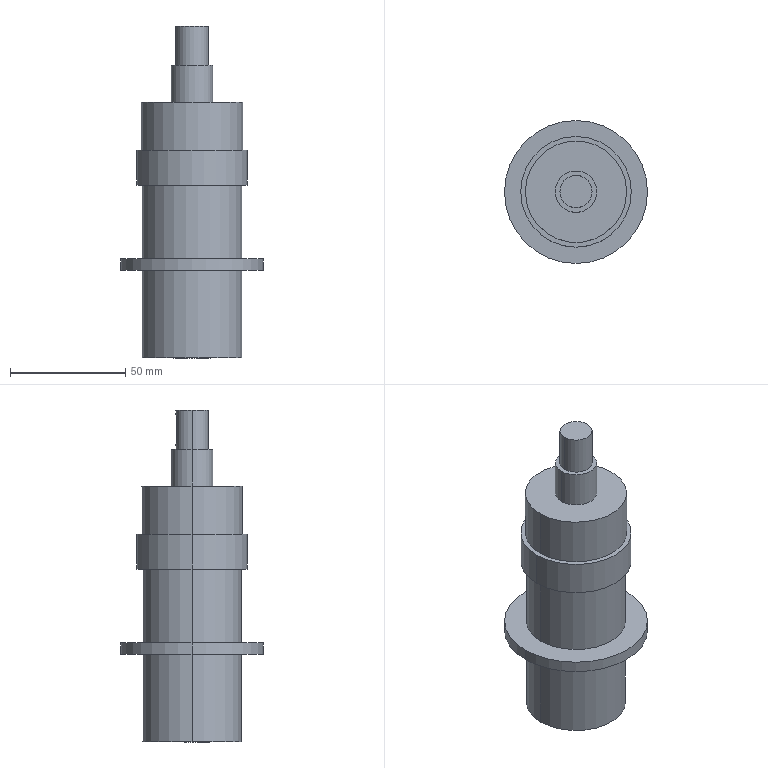Part | SolidWorks | features ICE 6, 3DProfileFeature 1, Cut 1, Extrusion 1, HoleWzd 1 | 1 solid | 32 faces | box 62 x 62 x 144 mm | volume 181126 mm3 | cylinder 19 | plane 11 | cone 2 | commonest cylinder face diameters 43 x4 3.7 x3 6.8 x2 14 x2 18 x2 44 x2
STEP:
#1=CARTESIAN_POINT('',(3.4,0.,35.));
#2=VERTEX_POINT('',#1);
#3=CARTESIAN_POINT('',(-3.4,0.,35.));
#4=VERTEX_POINT('',#3);
#5=CARTESIAN_POINT('',(0.,0.,35.));
#6=DIRECTION('',(0.,0.,-1.));
#7=DIRECTION('',(-1.,0.,0.));
#8=AXIS2_PLACEMENT_3D('',#5,#6,#7);
#9=CIRCLE('',#8,3.4);
#10=EDGE_CURVE('',#2,#4,#9,.T.);
#11=ORIENTED_EDGE('',*,*,#10,.F.);
#12=CARTESIAN_POINT('',(3.4,0.,0.));
#13=VERTEX_POINT('',#12);
#14=CARTESIAN_POINT('',(3.4,0.,0.));
#15=DIRECTION('',(0.,0.,-1.));
#16=VECTOR('',#15,1000.);
#17=LINE('',#14,#16);
#18=EDGE_CURVE('',#2,#13,#17,.T.);
#19=ORIENTED_EDGE('',*,*,#18,.T.);
#20=CARTESIAN_POINT('',(-3.4,0.,0.));
#21=VERTEX_POINT('',#20);
#22=CARTESIAN_POINT('',(0.,0.,0.));
#23=DIRECTION('',(0.,0.,-1.));
#24=DIRECTION('',(-1.,0.,0.));
#25=AXIS2_PLACEMENT_3D('',#22,#23,#24);
#26=CIRCLE('',#25,3.4);
#27=EDGE_CURVE('',#13,#21,#26,.T.);
#28=ORIENTED_EDGE('',*,*,#27,.T.);
#29=CARTESIAN_POINT('',(-3.4,0.,0.));
#30=DIRECTION('',(0.,0.,-1.));
#31=VECTOR('',#30,1000.);
#32=LINE('',#29,#31);
#33=EDGE_CURVE('',#4,#21,#32,.T.);
#34=ORIENTED_EDGE('',*,*,#33,.F.);
#35=EDGE_LOOP('',(#11,#19,#28,#34));
#36=FACE_OUTER_BOUND('',#35,.T.);
#37=CARTESIAN_POINT('',(0.,0.,0.));
#38=DIRECTION('',(0.,0.,-1.));
#39=DIRECTION('',(-1.,0.,0.));
#40=AXIS2_PLACEMENT_3D('',#37,#38,#39);
#41=CYLINDRICAL_SURFACE('',#40,3.4);
#42=ADVANCED_FACE('',(#36),#41,.F.);
#43=CARTESIAN_POINT('',(0.,0.,37.043));
#44=VERTEX_POINT('',#43);
#45=CARTESIAN_POINT('',(-3.4,0.,35.));
#46=DIRECTION('',(-0.8572,0.,-0.515));
#47=VECTOR('',#46,1000.);
#48=LINE('',#45,#47);
#49=EDGE_CURVE('',#44,#4,#48,.T.);
#50=ORIENTED_EDGE('',*,*,#49,.F.);
#51=CARTESIAN_POINT('',(3.4,0.,35.));
#52=DIRECTION('',(0.8572,0.,-0.515));
#53=VECTOR('',#52,1000.);
#54=LINE('',#51,#53);
#55=EDGE_CURVE('',#44,#2,#54,.T.);
#56=ORIENTED_EDGE('',*,*,#55,.T.);
#57=ORIENTED_EDGE('',*,*,#10,.T.);
#58=EDGE_LOOP('',(#50,#56,#57));
#59=FACE_OUTER_BOUND('',#58,.T.);
#60=CARTESIAN_POINT('',(0.,0.,35.));
#61=DIRECTION('',(0.,0.,-1.));
#62=DIRECTION('',(-1.,0.,0.));
#63=AXIS2_PLACEMENT_3D('',#60,#61,#62);
#64=CONICAL_SURFACE('',#63,3.4,1.03);
#65=ADVANCED_FACE('',(#59),#64,.F.);
#66=CARTESIAN_POINT('',(21.5,0.,38.));
#67=VERTEX_POINT('',#66);
#68=CARTESIAN_POINT('',(-21.5,0.,38.));
#69=VERTEX_POINT('',#68);
#70=CARTESIAN_POINT('',(0.,0.,38.));
#71=DIRECTION('',(0.,0.,1.));
#72=DIRECTION('',(1.,0.,0.));
#73=AXIS2_PLACEMENT_3D('',#70,#71,#72);
#74=CIRCLE('',#73,21.5);
#75=EDGE_CURVE('',#67,#69,#74,.T.);
#76=ORIENTED_EDGE('',*,*,#75,.F.);
#77=CARTESIAN_POINT('',(21.5,0.,0.));
#78=VERTEX_POINT('',#77);
#79=CARTESIAN_POINT('',(21.5,0.,75.));
#80=DIRECTION('',(0.,0.,-1.));
#81=VECTOR('',#80,1000.);
#82=LINE('',#79,#81);
#83=EDGE_CURVE('',#67,#78,#82,.T.);
#84=ORIENTED_EDGE('',*,*,#83,.T.);
#85=CARTESIAN_POINT('',(-21.5,0.,0.));
#86=VERTEX_POINT('',#85);
#87=CARTESIAN_POINT('',(0.,0.,0.));
#88=DIRECTION('',(0.,0.,-1.));
#89=DIRECTION('',(-1.,0.,0.));
#90=AXIS2_PLACEMENT_3D('',#87,#88,#89);
#91=CIRCLE('',#90,21.5);
#92=EDGE_CURVE('',#86,#78,#91,.T.);
#93=ORIENTED_EDGE('',*,*,#92,.F.);
#94=CARTESIAN_POINT('',(-21.5,0.,75.));
#95=DIRECTION('',(0.,0.,-1.));
#96=VECTOR('',#95,1000.);
#97=LINE('',#94,#96);
#98=EDGE_CURVE('',#69,#86,#97,.T.);
#99=ORIENTED_EDGE('',*,*,#98,.F.);
#100=EDGE_LOOP('',(#76,#84,#93,#99));
#101=FACE_OUTER_BOUND('',#100,.T.);
#102=CARTESIAN_POINT('',(0.,0.,75.));
#103=DIRECTION('',(0.,0.,-1.));
#104=DIRECTION('',(-1.,0.,0.));
#105=AXIS2_PLACEMENT_3D('',#102,#103,#104);
#106=CYLINDRICAL_SURFACE('',#105,21.5);
#107=ADVANCED_FACE('',(#101),#106,.T.);
#108=CARTESIAN_POINT('',(31.,0.,43.));
#109=VERTEX_POINT('',#108);
#110=CARTESIAN_POINT('',(-31.,0.,43.));
#111=VERTEX_POINT('',#110);
#112=CARTESIAN_POINT('',(0.,0.,43.));
#113=DIRECTION('',(0.,0.,1.));
#114=DIRECTION('',(1.,0.,0.));
#115=AXIS2_PLACEMENT_3D('',#112,#113,#114);
#116=CIRCLE('',#115,31.);
#117=EDGE_CURVE('',#109,#111,#116,.T.);
#118=ORIENTED_EDGE('',*,*,#117,.F.);
#119=CARTESIAN_POINT('',(31.,0.,38.));
#120=VERTEX_POINT('',#119);
#121=CARTESIAN_POINT('',(31.,0.,43.));
#122=DIRECTION('',(0.,0.,-1.));
#123=VECTOR('',#122,1000.);
#124=LINE('',#121,#123);
#125=EDGE_CURVE('',#109,#120,#124,.T.);
#126=ORIENTED_EDGE('',*,*,#125,.T.);
#127=CARTESIAN_POINT('',(-31.,0.,38.));
#128=VERTEX_POINT('',#127);
#129=CARTESIAN_POINT('',(0.,0.,38.));
#130=DIRECTION('',(0.,0.,1.));
#131=DIRECTION('',(1.,0.,0.));
#132=AXIS2_PLACEMENT_3D('',#129,#130,#131);
#133=CIRCLE('',#132,31.);
#134=EDGE_CURVE('',#120,#128,#133,.T.);
#135=ORIENTED_EDGE('',*,*,#134,.T.);
#136=CARTESIAN_POINT('',(-31.,0.,43.));
#137=DIRECTION('',(0.,0.,-1.));
#138=VECTOR('',#137,1000.);
#139=LINE('',#136,#138);
#140=EDGE_CURVE('',#111,#128,#139,.T.);
#141=ORIENTED_EDGE('',*,*,#140,.F.);
#142=EDGE_LOOP('',(#118,#126,#135,#141));
#143=FACE_OUTER_BOUND('',#142,.T.);
#144=CARTESIAN_POINT('',(0.,0.,43.));
#145=DIRECTION('',(0.,0.,-1.));
#146=DIRECTION('',(-1.,0.,0.));
#147=AXIS2_PLACEMENT_3D('',#144,#145,#146);
#148=CYLINDRICAL_SURFACE('',#147,31.);
#149=ADVANCED_FACE('',(#143),#148,.T.);
#150=CARTESIAN_POINT('',(0.,5.,142.35));
#151=VERTEX_POINT('',#150);
#152=CARTESIAN_POINT('',(1.85,5.,140.5));
#153=VERTEX_POINT('',#152);
#154=CARTESIAN_POINT('',(0.,5.,140.5));
#155=DIRECTION('',(0.,1.,0.));
#156=DIRECTION('',(0.,0.,1.));
#157=AXIS2_PLACEMENT_3D('',#154,#155,#156);
#158=CIRCLE('',#157,1.85);
#159=EDGE_CURVE('',#151,#153,#158,.T.);
#160=ORIENTED_EDGE('',*,*,#159,.F.);
#161=CARTESIAN_POINT('',(0.,7.,142.35));
#162=VERTEX_POINT('',#161);
#163=CARTESIAN_POINT('',(0.,5.,142.35));
#164=DIRECTION('',(0.,1.,0.));
#165=VECTOR('',#164,1000.);
#166=LINE('',#163,#165);
#167=EDGE_CURVE('',#151,#162,#166,.T.);
#168=ORIENTED_EDGE('',*,*,#167,.T.);
#169=CARTESIAN_POINT('',(1.85,6.751,140.5));
#170=VERTEX_POINT('',#169);
#171=CARTESIAN_POINT('',(1.85,6.751,140.5));
#172=CARTESIAN_POINT('',(1.85,6.751,140.623));
#173=CARTESIAN_POINT('',(1.838,6.754,140.744));
#174=CARTESIAN_POINT('',(1.791,6.767,140.981));
#175=CARTESIAN_POINT('',(1.755,6.777,141.099));
#176=CARTESIAN_POINT('',(1.662,6.8,141.322));
#177=CARTESIAN_POINT('',(1.605,6.814,141.429));
#178=CARTESIAN_POINT('',(1.47,6.844,141.629));
#179=CARTESIAN_POINT('',(1.393,6.861,141.724));
#180=CARTESIAN_POINT('',(1.138,6.909,141.979));
#181=CARTESIAN_POINT('',(0.932,6.941,142.116));
#182=CARTESIAN_POINT('',(0.5982,6.975,142.255));
#183=CARTESIAN_POINT('',(0.4809,6.984,142.291));
#184=CARTESIAN_POINT('',(0.2418,6.997,142.338));
#185=CARTESIAN_POINT('',(0.1213,7.,142.35));
#186=CARTESIAN_POINT('',(0.,7.,142.35));
#187=B_SPLINE_CURVE_WITH_KNOTS('',3,(#171,#172,#173,#174,#175,#176,#177,#178,#179,#180,#181,#182,#183,#184,#185,#186),.UNSPECIFIED.,.F.,.F.,(4,2,2,2,2,2,2,4),(0.,0.0003632,0.0007264,0.00109,0.001453,0.002179,0.002542,0.002906),.UNSPECIFIED.);
#188=EDGE_CURVE('',#170,#162,#187,.T.);
#189=ORIENTED_EDGE('',*,*,#188,.F.);
#190=CARTESIAN_POINT('',(1.85,5.,140.5));
#191=DIRECTION('',(0.,1.,0.));
#192=VECTOR('',#191,1000.);
#193=LINE('',#190,#192);
#194=EDGE_CURVE('',#153,#170,#193,.T.);
#195=ORIENTED_EDGE('',*,*,#194,.F.);
#196=EDGE_LOOP('',(#160,#168,#189,#195));
#197=FACE_OUTER_BOUND('',#196,.T.);
#198=CARTESIAN_POINT('',(0.,5.,140.5));
#199=DIRECTION('',(0.,1.,0.));
#200=DIRECTION('',(0.,0.,1.));
#201=AXIS2_PLACEMENT_3D('',#198,#199,#200);
#202=CYLINDRICAL_SURFACE('',#201,1.85);
#203=ADVANCED_FACE('',(#197),#202,.F.);
#204=CARTESIAN_POINT('',(-1.85,6.751,140.5));
#205=VERTEX_POINT('',#204);
#206=CARTESIAN_POINT('',(-1.85,6.751,130.64));
#207=VERTEX_POINT('',#206);
#208=CARTESIAN_POINT('',(-1.85,6.751,144.));
#209=DIRECTION('',(0.,0.,-1.));
#210=VECTOR('',#209,1000.);
#211=LINE('',#208,#210);
#212=EDGE_CURVE('',#205,#207,#211,.T.);
#213=ORIENTED_EDGE('',*,*,#212,.T.);
#214=CARTESIAN_POINT('',(1.85,6.751,130.64));
#215=VERTEX_POINT('',#214);
#216=CARTESIAN_POINT('',(-1.85,6.751,130.64));
#217=CARTESIAN_POINT('',(-1.85,6.751,130.517));
#218=CARTESIAN_POINT('',(-1.838,6.754,130.397));
#219=CARTESIAN_POINT('',(-1.791,6.767,130.159));
#220=CARTESIAN_POINT('',(-1.755,6.777,130.042));
#221=CARTESIAN_POINT('',(-1.662,6.8,129.818));
#222=CARTESIAN_POINT('',(-1.605,6.814,129.712));
#223=CARTESIAN_POINT('',(-1.471,6.844,129.511));
#224=CARTESIAN_POINT('',(-1.393,6.861,129.417));
#225=CARTESIAN_POINT('',(-1.138,6.909,129.162));
#226=CARTESIAN_POINT('',(-0.933,6.941,129.024));
#227=CARTESIAN_POINT('',(-0.5995,6.975,128.886));
#228=CARTESIAN_POINT('',(-0.4823,6.984,128.85));
#229=CARTESIAN_POINT('',(-0.2433,6.997,128.802));
#230=CARTESIAN_POINT('',(-0.1229,7.,128.79));
#231=CARTESIAN_POINT('',(0.1195,7.,128.79));
#232=CARTESIAN_POINT('',(0.2427,6.997,128.802));
#233=CARTESIAN_POINT('',(0.4804,6.985,128.849));
#234=CARTESIAN_POINT('',(0.596,6.975,128.884));
#235=CARTESIAN_POINT('',(0.933,6.941,129.024));
#236=CARTESIAN_POINT('',(1.136,6.909,129.16));
#237=CARTESIAN_POINT('',(1.393,6.86,129.417));
#238=CARTESIAN_POINT('',(1.469,6.844,129.51));
#239=CARTESIAN_POINT('',(1.603,6.814,129.709));
#240=CARTESIAN_POINT('',(1.662,6.8,129.818));
#241=CARTESIAN_POINT('',(1.801,6.765,130.152));
#242=CARTESIAN_POINT('',(1.85,6.751,130.394));
#243=CARTESIAN_POINT('',(1.85,6.751,130.64));
#244=B_SPLINE_CURVE_WITH_KNOTS('',3,(#216,#217,#218,#219,#220,#221,#222,#223,#224,#225,#226,#227,#228,#229,#230,#231,#232,#233,#234,#235,#236,#237,#238,#239,#240,#241,#242,#243),.UNSPECIFIED.,.F.,.F.,(4,2,2,2,2,2,2,2,2,2,2,2,2,4),(0.,0.000363,0.000726,0.001089,0.001452,0.002178,0.002541,0.002904,0.003267,0.00363,0.004356,0.004719,0.005082,0.005808),.UNSPECIFIED.);
#245=EDGE_CURVE('',#207,#215,#244,.T.);
#246=ORIENTED_EDGE('',*,*,#245,.T.);
#247=CARTESIAN_POINT('',(1.85,6.751,144.));
#248=DIRECTION('',(0.,0.,1.));
#249=VECTOR('',#248,1000.);
#250=LINE('',#247,#249);
#251=EDGE_CURVE('',#215,#170,#250,.T.);
#252=ORIENTED_EDGE('',*,*,#251,.T.);
#253=ORIENTED_EDGE('',*,*,#188,.T.);
#254=CARTESIAN_POINT('',(0.,7.,142.35));
#255=CARTESIAN_POINT('',(-0.1212,7.,142.35));
#256=CARTESIAN_POINT('',(-0.2443,6.997,142.338));
#257=CARTESIAN_POINT('',(-0.4818,6.984,142.29));
#258=CARTESIAN_POINT('',(-0.5973,6.975,142.255));
#259=CARTESIAN_POINT('',(-0.934,6.941,142.115));
#260=CARTESIAN_POINT('',(-1.137,6.909,141.979));
#261=CARTESIAN_POINT('',(-1.394,6.86,141.723));
#262=CARTESIAN_POINT('',(-1.47,6.844,141.63));
#263=CARTESIAN_POINT('',(-1.604,6.814,141.43));
#264=CARTESIAN_POINT('',(-1.662,6.8,141.322));
#265=CARTESIAN_POINT('',(-1.801,6.765,140.987));
#266=CARTESIAN_POINT('',(-1.85,6.751,140.745));
#267=CARTESIAN_POINT('',(-1.85,6.751,140.5));
#268=B_SPLINE_CURVE_WITH_KNOTS('',3,(#254,#255,#256,#257,#258,#259,#260,#261,#262,#263,#264,#265,#266,#267),.UNSPECIFIED.,.F.,.F.,(4,2,2,2,2,2,4),(0.002906,0.003268,0.003631,0.004357,0.00472,0.005082,0.005808),.UNSPECIFIED.);
#269=EDGE_CURVE('',#162,#205,#268,.T.);
#270=ORIENTED_EDGE('',*,*,#269,.T.);
#271=EDGE_LOOP('',(#213,#246,#252,#253,#270));
#272=FACE_BOUND('',#271,.T.);
#273=CARTESIAN_POINT('',(7.,0.,144.));
#274=VERTEX_POINT('',#273);
#275=CARTESIAN_POINT('',(-7.,0.,144.));
#276=VERTEX_POINT('',#275);
#277=CARTESIAN_POINT('',(0.,0.,144.));
#278=DIRECTION('',(0.,0.,1.));
#279=DIRECTION('',(1.,0.,0.));
#280=AXIS2_PLACEMENT_3D('',#277,#278,#279);
#281=CIRCLE('',#280,7.);
#282=EDGE_CURVE('',#274,#276,#281,.T.);
#283=ORIENTED_EDGE('',*,*,#282,.F.);
#284=CARTESIAN_POINT('',(7.,0.,127.));
#285=VERTEX_POINT('',#284);
#286=CARTESIAN_POINT('',(7.,0.,144.));
#287=DIRECTION('',(0.,0.,-1.));
#288=VECTOR('',#287,1000.);
#289=LINE('',#286,#288);
#290=EDGE_CURVE('',#274,#285,#289,.T.);
#291=ORIENTED_EDGE('',*,*,#290,.T.);
#292=CARTESIAN_POINT('',(-7.,0.,127.));
#293=VERTEX_POINT('',#292);
#294=CARTESIAN_POINT('',(0.,0.,127.));
#295=DIRECTION('',(0.,0.,1.));
#296=DIRECTION('',(1.,0.,0.));
#297=AXIS2_PLACEMENT_3D('',#294,#295,#296);
#298=CIRCLE('',#297,7.);
#299=EDGE_CURVE('',#285,#293,#298,.T.);
#300=ORIENTED_EDGE('',*,*,#299,.T.);
#301=CARTESIAN_POINT('',(-7.,0.,144.));
#302=DIRECTION('',(0.,0.,-1.));
#303=VECTOR('',#302,1000.);
#304=LINE('',#301,#303);
#305=EDGE_CURVE('',#276,#293,#304,.T.);
#306=ORIENTED_EDGE('',*,*,#305,.F.);
#307=EDGE_LOOP('',(#283,#291,#300,#306));
#308=FACE_OUTER_BOUND('',#307,.T.);
#309=CARTESIAN_POINT('',(0.,0.,144.));
#310=DIRECTION('',(0.,0.,-1.));
#311=DIRECTION('',(-1.,0.,0.));
#312=AXIS2_PLACEMENT_3D('',#309,#310,#311);
#313=CYLINDRICAL_SURFACE('',#312,7.);
#314=ADVANCED_FACE('',(#272,#308),#313,.T.);
#315=CARTESIAN_POINT('',(9.,0.,127.));
#316=VERTEX_POINT('',#315);
#317=CARTESIAN_POINT('',(-9.,0.,127.));
#318=VERTEX_POINT('',#317);
#319=CARTESIAN_POINT('',(0.,0.,127.));
#320=DIRECTION('',(0.,0.,1.));
#321=DIRECTION('',(1.,0.,0.));
#322=AXIS2_PLACEMENT_3D('',#319,#320,#321);
#323=CIRCLE('',#322,9.);
#324=EDGE_CURVE('',#316,#318,#323,.T.);
#325=ORIENTED_EDGE('',*,*,#324,.F.);
#326=CARTESIAN_POINT('',(9.,0.,111.));
#327=VERTEX_POINT('',#326);
#328=CARTESIAN_POINT('',(9.,0.,127.));
#329=DIRECTION('',(0.,0.,-1.));
#330=VECTOR('',#329,1000.);
#331=LINE('',#328,#330);
#332=EDGE_CURVE('',#316,#327,#331,.T.);
#333=ORIENTED_EDGE('',*,*,#332,.T.);
#334=CARTESIAN_POINT('',(-9.,0.,111.));
#335=VERTEX_POINT('',#334);
#336=CARTESIAN_POINT('',(0.,0.,111.));
#337=DIRECTION('',(0.,0.,1.));
#338=DIRECTION('',(1.,0.,0.));
#339=AXIS2_PLACEMENT_3D('',#336,#337,#338);
#340=CIRCLE('',#339,9.);
#341=EDGE_CURVE('',#327,#335,#340,.T.);
#342=ORIENTED_EDGE('',*,*,#341,.T.);
#343=CARTESIAN_POINT('',(-9.,0.,127.));
#344=DIRECTION('',(0.,0.,-1.));
#345=VECTOR('',#344,1000.);
#346=LINE('',#343,#345);
#347=EDGE_CURVE('',#318,#335,#346,.T.);
#348=ORIENTED_EDGE('',*,*,#347,.F.);
#349=EDGE_LOOP('',(#325,#333,#342,#348));
#350=FACE_OUTER_BOUND('',#349,.T.);
#351=CARTESIAN_POINT('',(0.,0.,127.));
#352=DIRECTION('',(0.,0.,-1.));
#353=DIRECTION('',(-1.,0.,0.));
#354=AXIS2_PLACEMENT_3D('',#351,#352,#353);
#355=CYLINDRICAL_SURFACE('',#354,9.);
#356=ADVANCED_FACE('',(#350),#355,.T.);
#357=CARTESIAN_POINT('',(22.,0.,111.));
#358=VERTEX_POINT('',#357);
#359=CARTESIAN_POINT('',(-22.,0.,111.));
#360=VERTEX_POINT('',#359);
#361=CARTESIAN_POINT('',(0.,0.,111.));
#362=DIRECTION('',(0.,0.,1.));
#363=DIRECTION('',(1.,0.,0.));
#364=AXIS2_PLACEMENT_3D('',#361,#362,#363);
#365=CIRCLE('',#364,22.);
#366=EDGE_CURVE('',#358,#360,#365,.T.);
#367=ORIENTED_EDGE('',*,*,#366,.F.);
#368=CARTESIAN_POINT('',(22.,0.,90.));
#369=VERTEX_POINT('',#368);
#370=CARTESIAN_POINT('',(22.,0.,111.));
#371=DIRECTION('',(0.,0.,-1.));
#372=VECTOR('',#371,1000.);
#373=LINE('',#370,#372);
#374=EDGE_CURVE('',#358,#369,#373,.T.);
#375=ORIENTED_EDGE('',*,*,#374,.T.);
#376=CARTESIAN_POINT('',(-22.,0.,90.));
#377=VERTEX_POINT('',#376);
#378=CARTESIAN_POINT('',(0.,0.,90.));
#379=DIRECTION('',(0.,0.,1.));
#380=DIRECTION('',(1.,0.,0.));
#381=AXIS2_PLACEMENT_3D('',#378,#379,#380);
#382=CIRCLE('',#381,22.);
#383=EDGE_CURVE('',#369,#377,#382,.T.);
#384=ORIENTED_EDGE('',*,*,#383,.T.);
#385=CARTESIAN_POINT('',(-22.,0.,111.));
#386=DIRECTION('',(0.,0.,-1.));
#387=VECTOR('',#386,1000.);
#388=LINE('',#385,#387);
#389=EDGE_CURVE('',#360,#377,#388,.T.);
#390=ORIENTED_EDGE('',*,*,#389,.F.);
#391=EDGE_LOOP('',(#367,#375,#384,#390));
#392=FACE_OUTER_BOUND('',#391,.T.);
#393=CARTESIAN_POINT('',(0.,0.,111.));
#394=DIRECTION('',(0.,0.,-1.));
#395=DIRECTION('',(-1.,0.,0.));
#396=AXIS2_PLACEMENT_3D('',#393,#394,#395);
#397=CYLINDRICAL_SURFACE('',#396,22.);
#398=ADVANCED_FACE('',(#392),#397,.T.);
#399=CARTESIAN_POINT('',(24.,0.,90.));
#400=VERTEX_POINT('',#399);
#401=CARTESIAN_POINT('',(-24.,0.,90.));
#402=VERTEX_POINT('',#401);
#403=CARTESIAN_POINT('',(0.,0.,90.));
#404=DIRECTION('',(0.,0.,1.));
#405=DIRECTION('',(1.,0.,0.));
#406=AXIS2_PLACEMENT_3D('',#403,#404,#405);
#407=CIRCLE('',#406,24.);
#408=EDGE_CURVE('',#400,#402,#407,.T.);
#409=ORIENTED_EDGE('',*,*,#408,.F.);
#410=CARTESIAN_POINT('',(24.,0.,75.));
#411=VERTEX_POINT('',#410);
#412=CARTESIAN_POINT('',(24.,0.,90.));
#413=DIRECTION('',(0.,0.,-1.));
#414=VECTOR('',#413,1000.);
#415=LINE('',#412,#414);
#416=EDGE_CURVE('',#400,#411,#415,.T.);
#417=ORIENTED_EDGE('',*,*,#416,.T.);
#418=CARTESIAN_POINT('',(-24.,0.,75.));
#419=VERTEX_POINT('',#418);
#420=CARTESIAN_POINT('',(0.,0.,75.));
#421=DIRECTION('',(0.,0.,1.));
#422=DIRECTION('',(1.,0.,0.));
#423=AXIS2_PLACEMENT_3D('',#420,#421,#422);
#424=CIRCLE('',#423,24.);
#425=EDGE_CURVE('',#411,#419,#424,.T.);
#426=ORIENTED_EDGE('',*,*,#425,.T.);
#427=CARTESIAN_POINT('',(-24.,0.,90.));
#428=DIRECTION('',(0.,0.,-1.));
#429=VECTOR('',#428,1000.);
#430=LINE('',#427,#429);
#431=EDGE_CURVE('',#402,#419,#430,.T.);
#432=ORIENTED_EDGE('',*,*,#431,.F.);
#433=EDGE_LOOP('',(#409,#417,#426,#432));
#434=FACE_OUTER_BOUND('',#433,.T.);
#435=CARTESIAN_POINT('',(0.,0.,90.));
#436=DIRECTION('',(0.,0.,-1.));
#437=DIRECTION('',(-1.,0.,0.));
#438=AXIS2_PLACEMENT_3D('',#435,#436,#437);
#439=CYLINDRICAL_SURFACE('',#438,24.);
#440=ADVANCED_FACE('',(#434),#439,.T.);
#441=CARTESIAN_POINT('',(21.5,0.,75.));
#442=VERTEX_POINT('',#441);
#443=CARTESIAN_POINT('',(-21.5,0.,75.));
#444=VERTEX_POINT('',#443);
#445=CARTESIAN_POINT('',(0.,0.,75.));
#446=DIRECTION('',(0.,0.,1.));
#447=DIRECTION('',(1.,0.,0.));
#448=AXIS2_PLACEMENT_3D('',#445,#446,#447);
#449=CIRCLE('',#448,21.5);
#450=EDGE_CURVE('',#442,#444,#449,.T.);
#451=ORIENTED_EDGE('',*,*,#450,.F.);
#452=CARTESIAN_POINT('',(21.5,0.,43.));
#453=VERTEX_POINT('',#452);
#454=CARTESIAN_POINT('',(21.5,0.,75.));
#455=DIRECTION('',(0.,0.,-1.));
#456=VECTOR('',#455,1000.);
#457=LINE('',#454,#456);
#458=EDGE_CURVE('',#442,#453,#457,.T.);
#459=ORIENTED_EDGE('',*,*,#458,.T.);
#460=CARTESIAN_POINT('',(-21.5,0.,43.));
#461=VERTEX_POINT('',#460);
#462=CARTESIAN_POINT('',(0.,0.,43.));
#463=DIRECTION('',(0.,0.,1.));
#464=DIRECTION('',(1.,0.,0.));
#465=AXIS2_PLACEMENT_3D('',#462,#463,#464);
#466=CIRCLE('',#465,21.5);
#467=EDGE_CURVE('',#453,#461,#466,.T.);
#468=ORIENTED_EDGE('',*,*,#467,.T.);
#469=CARTESIAN_POINT('',(-21.5,0.,75.));
#470=DIRECTION('',(0.,0.,-1.));
#471=VECTOR('',#470,1000.);
#472=LINE('',#469,#471);
#473=EDGE_CURVE('',#444,#461,#472,.T.);
#474=ORIENTED_EDGE('',*,*,#473,.F.);
#475=EDGE_LOOP('',(#451,#459,#468,#474));
#476=FACE_OUTER_BOUND('',#475,.T.);
#477=CARTESIAN_POINT('',(0.,0.,75.));
#478=DIRECTION('',(0.,0.,-1.));
#479=DIRECTION('',(-1.,0.,0.));
#480=AXIS2_PLACEMENT_3D('',#477,#478,#479);
#481=CYLINDRICAL_SURFACE('',#480,21.5);
#482=ADVANCED_FACE('',(#476),#481,.T.);
#483=ORIENTED_EDGE('',*,*,#458,.F.);
#484=CARTESIAN_POINT('',(0.,0.,75.));
#485=DIRECTION('',(0.,0.,1.));
#486=DIRECTION('',(1.,0.,0.));
#487=AXIS2_PLACEMENT_3D('',#484,#485,#486);
#488=CIRCLE('',#487,21.5);
#489=EDGE_CURVE('',#444,#442,#488,.T.);
#490=ORIENTED_EDGE('',*,*,#489,.F.);
#491=ORIENTED_EDGE('',*,*,#473,.T.);
#492=CARTESIAN_POINT('',(0.,0.,43.));
#493=DIRECTION('',(0.,0.,1.));
#494=DIRECTION('',(1.,0.,0.));
#495=AXIS2_PLACEMENT_3D('',#492,#493,#494);
#496=CIRCLE('',#495,21.5);
#497=EDGE_CURVE('',#461,#453,#496,.T.);
#498=ORIENTED_EDGE('',*,*,#497,.T.);
#499=EDGE_LOOP('',(#483,#490,#491,#498));
#500=FACE_OUTER_BOUND('',#499,.T.);
#501=CARTESIAN_POINT('',(0.,0.,75.));
#502=DIRECTION('',(0.,0.,-1.));
#503=DIRECTION('',(-1.,0.,0.));
#504=AXIS2_PLACEMENT_3D('',#501,#502,#503);
#505=CYLINDRICAL_SURFACE('',#504,21.5);
#506=ADVANCED_FACE('',(#500),#505,.T.);
#507=ORIENTED_EDGE('',*,*,#416,.F.);
#508=CARTESIAN_POINT('',(0.,0.,90.));
#509=DIRECTION('',(0.,0.,1.));
#510=DIRECTION('',(1.,0.,0.));
#511=AXIS2_PLACEMENT_3D('',#508,#509,#510);
#512=CIRCLE('',#511,24.);
#513=EDGE_CURVE('',#402,#400,#512,.T.);
#514=ORIENTED_EDGE('',*,*,#513,.F.);
#515=ORIENTED_EDGE('',*,*,#431,.T.);
#516=CARTESIAN_POINT('',(0.,0.,75.));
#517=DIRECTION('',(0.,0.,1.));
#518=DIRECTION('',(1.,0.,0.));
#519=AXIS2_PLACEMENT_3D('',#516,#517,#518);
#520=CIRCLE('',#519,24.);
#521=EDGE_CURVE('',#419,#411,#520,.T.);
#522=ORIENTED_EDGE('',*,*,#521,.T.);
#523=EDGE_LOOP('',(#507,#514,#515,#522));
#524=FACE_OUTER_BOUND('',#523,.T.);
#525=CARTESIAN_POINT('',(0.,0.,90.));
#526=DIRECTION('',(0.,0.,-1.));
#527=DIRECTION('',(-1.,0.,0.));
#528=AXIS2_PLACEMENT_3D('',#525,#526,#527);
#529=CYLINDRICAL_SURFACE('',#528,24.);
#530=ADVANCED_FACE('',(#524),#529,.T.);
#531=CARTESIAN_POINT('',(0.,0.,90.));
#532=DIRECTION('',(0.,0.,1.));
#533=DIRECTION('',(1.,0.,0.));
#534=AXIS2_PLACEMENT_3D('',#531,#532,#533);
#535=CIRCLE('',#534,22.);
#536=EDGE_CURVE('',#377,#369,#535,.T.);
#537=ORIENTED_EDGE('',*,*,#536,.F.);
#538=ORIENTED_EDGE('',*,*,#383,.F.);
#539=EDGE_LOOP('',(#537,#538));
#540=FACE_BOUND('',#539,.T.);
#541=ORIENTED_EDGE('',*,*,#513,.T.);
#542=ORIENTED_EDGE('',*,*,#408,.T.);
#543=EDGE_LOOP('',(#541,#542));
#544=FACE_OUTER_BOUND('',#543,.T.);
#545=CARTESIAN_POINT('',(0.,0.,90.));
#546=DIRECTION('',(0.,0.,1.));
#547=DIRECTION('',(1.,0.,0.));
#548=AXIS2_PLACEMENT_3D('',#545,#546,#547);
#549=PLANE('',#548);
#550=ADVANCED_FACE('',(#540,#544),#549,.T.);
#551=ORIENTED_EDGE('',*,*,#489,.T.);
#552=ORIENTED_EDGE('',*,*,#450,.T.);
#553=EDGE_LOOP('',(#551,#552));
#554=FACE_BOUND('',#553,.T.);
#555=ORIENTED_EDGE('',*,*,#521,.F.);
#556=ORIENTED_EDGE('',*,*,#425,.F.);
#557=EDGE_LOOP('',(#555,#556));
#558=FACE_OUTER_BOUND('',#557,.T.);
#559=CARTESIAN_POINT('',(0.,0.,75.));
#560=DIRECTION('',(0.,0.,1.));
#561=DIRECTION('',(1.,0.,0.));
#562=AXIS2_PLACEMENT_3D('',#559,#560,#561);
#563=PLANE('',#562);
#564=ADVANCED_FACE('',(#554,#558),#563,.F.);
#565=ORIENTED_EDGE('',*,*,#374,.F.);
#566=CARTESIAN_POINT('',(0.,0.,111.));
#567=DIRECTION('',(0.,0.,1.));
#568=DIRECTION('',(1.,0.,0.));
#569=AXIS2_PLACEMENT_3D('',#566,#567,#568);
#570=CIRCLE('',#569,22.);
#571=EDGE_CURVE('',#360,#358,#570,.T.);
#572=ORIENTED_EDGE('',*,*,#571,.F.);
#573=ORIENTED_EDGE('',*,*,#389,.T.);
#574=ORIENTED_EDGE('',*,*,#536,.T.);
#575=EDGE_LOOP('',(#565,#572,#573,#574));
#576=FACE_OUTER_BOUND('',#575,.T.);
#577=CARTESIAN_POINT('',(0.,0.,111.));
#578=DIRECTION('',(0.,0.,-1.));
#579=DIRECTION('',(-1.,0.,0.));
#580=AXIS2_PLACEMENT_3D('',#577,#578,#579);
#581=CYLINDRICAL_SURFACE('',#580,22.);
#582=ADVANCED_FACE('',(#576),#581,.T.);
#583=CARTESIAN_POINT('',(0.,0.,111.));
#584=DIRECTION('',(0.,0.,1.));
#585=DIRECTION('',(1.,0.,0.));
#586=AXIS2_PLACEMENT_3D('',#583,#584,#585);
#587=CIRCLE('',#586,9.);
#588=EDGE_CURVE('',#335,#327,#587,.T.);
#589=ORIENTED_EDGE('',*,*,#588,.F.);
#590=ORIENTED_EDGE('',*,*,#341,.F.);
#591=EDGE_LOOP('',(#589,#590));
#592=FACE_BOUND('',#591,.T.);
#593=ORIENTED_EDGE('',*,*,#571,.T.);
#594=ORIENTED_EDGE('',*,*,#366,.T.);
#595=EDGE_LOOP('',(#593,#594));
#596=FACE_OUTER_BOUND('',#595,.T.);
#597=CARTESIAN_POINT('',(0.,0.,111.));
#598=DIRECTION('',(0.,0.,1.));
#599=DIRECTION('',(1.,0.,0.));
#600=AXIS2_PLACEMENT_3D('',#597,#598,#599);
#601=PLANE('',#600);
#602=ADVANCED_FACE('',(#592,#596),#601,.T.);
#603=ORIENTED_EDGE('',*,*,#332,.F.);
#604=CARTESIAN_POINT('',(0.,0.,127.));
#605=DIRECTION('',(0.,0.,1.));
#606=DIRECTION('',(1.,0.,0.));
#607=AXIS2_PLACEMENT_3D('',#604,#605,#606);
#608=CIRCLE('',#607,9.);
#609=EDGE_CURVE('',#318,#316,#608,.T.);
#610=ORIENTED_EDGE('',*,*,#609,.F.);
#611=ORIENTED_EDGE('',*,*,#347,.T.);
#612=ORIENTED_EDGE('',*,*,#588,.T.);
#613=EDGE_LOOP('',(#603,#610,#611,#612));
#614=FACE_OUTER_BOUND('',#613,.T.);
#615=CARTESIAN_POINT('',(0.,0.,127.));
#616=DIRECTION('',(0.,0.,-1.));
#617=DIRECTION('',(-1.,0.,0.));
#618=AXIS2_PLACEMENT_3D('',#615,#616,#617);
#619=CYLINDRICAL_SURFACE('',#618,9.);
#620=ADVANCED_FACE('',(#614),#619,.T.);
#621=CARTESIAN_POINT('',(0.,0.,127.));
#622=DIRECTION('',(0.,0.,1.));
#623=DIRECTION('',(1.,0.,0.));
#624=AXIS2_PLACEMENT_3D('',#621,#622,#623);
#625=CIRCLE('',#624,7.);
#626=EDGE_CURVE('',#293,#285,#625,.T.);
#627=ORIENTED_EDGE('',*,*,#626,.F.);
#628=ORIENTED_EDGE('',*,*,#299,.F.);
#629=EDGE_LOOP('',(#627,#628));
#630=FACE_BOUND('',#629,.T.);
#631=ORIENTED_EDGE('',*,*,#609,.T.);
#632=ORIENTED_EDGE('',*,*,#324,.T.);
#633=EDGE_LOOP('',(#631,#632));
#634=FACE_OUTER_BOUND('',#633,.T.);
#635=CARTESIAN_POINT('',(0.,0.,127.));
#636=DIRECTION('',(0.,0.,1.));
#637=DIRECTION('',(1.,0.,0.));
#638=AXIS2_PLACEMENT_3D('',#635,#636,#637);
#639=PLANE('',#638);
#640=ADVANCED_FACE('',(#630,#634),#639,.T.);
#641=ORIENTED_EDGE('',*,*,#290,.F.);
#642=CARTESIAN_POINT('',(0.,0.,144.));
#643=DIRECTION('',(0.,0.,1.));
#644=DIRECTION('',(1.,0.,0.));
#645=AXIS2_PLACEMENT_3D('',#642,#643,#644);
#646=CIRCLE('',#645,7.);
#647=EDGE_CURVE('',#276,#274,#646,.T.);
#648=ORIENTED_EDGE('',*,*,#647,.F.);
#649=ORIENTED_EDGE('',*,*,#305,.T.);
#650=ORIENTED_EDGE('',*,*,#626,.T.);
#651=EDGE_LOOP('',(#641,#648,#649,#650));
#652=FACE_OUTER_BOUND('',#651,.T.);
#653=CARTESIAN_POINT('',(0.,0.,144.));
#654=DIRECTION('',(0.,0.,-1.));
#655=DIRECTION('',(-1.,0.,0.));
#656=AXIS2_PLACEMENT_3D('',#653,#654,#655);
#657=CYLINDRICAL_SURFACE('',#656,7.);
#658=ADVANCED_FACE('',(#652),#657,.T.);
#659=ORIENTED_EDGE('',*,*,#647,.T.);
#660=ORIENTED_EDGE('',*,*,#282,.T.);
#661=EDGE_LOOP('',(#659,#660));
#662=FACE_OUTER_BOUND('',#661,.T.);
#663=CARTESIAN_POINT('',(0.,0.,144.));
#664=DIRECTION('',(0.,0.,1.));
#665=DIRECTION('',(1.,0.,0.));
#666=AXIS2_PLACEMENT_3D('',#663,#664,#665);
#667=PLANE('',#666);
#668=ADVANCED_FACE('',(#662),#667,.T.);
#669=CARTESIAN_POINT('',(-1.85,5.,130.64));
#670=VERTEX_POINT('',#669);
#671=CARTESIAN_POINT('',(-1.85,5.,130.64));
#672=DIRECTION('',(0.,1.,0.));
#673=VECTOR('',#672,1000.);
#674=LINE('',#671,#673);
#675=EDGE_CURVE('',#670,#207,#674,.T.);
#676=ORIENTED_EDGE('',*,*,#675,.F.);
#677=CARTESIAN_POINT('',(1.85,5.,130.64));
#678=VERTEX_POINT('',#677);
#679=CARTESIAN_POINT('',(0.,5.,130.64));
#680=DIRECTION('',(0.,1.,0.));
#681=DIRECTION('',(0.,0.,1.));
#682=AXIS2_PLACEMENT_3D('',#679,#680,#681);
#683=CIRCLE('',#682,1.85);
#684=EDGE_CURVE('',#678,#670,#683,.T.);
#685=ORIENTED_EDGE('',*,*,#684,.F.);
#686=CARTESIAN_POINT('',(1.85,5.,130.64));
#687=DIRECTION('',(0.,1.,0.));
#688=VECTOR('',#687,1000.);
#689=LINE('',#686,#688);
#690=EDGE_CURVE('',#678,#215,#689,.T.);
#691=ORIENTED_EDGE('',*,*,#690,.T.);
#692=ORIENTED_EDGE('',*,*,#245,.F.);
#693=EDGE_LOOP('',(#676,#685,#691,#692));
#694=FACE_OUTER_BOUND('',#693,.T.);
#695=CARTESIAN_POINT('',(0.,5.,130.64));
#696=DIRECTION('',(0.,1.,0.));
#697=DIRECTION('',(0.,0.,1.));
#698=AXIS2_PLACEMENT_3D('',#695,#696,#697);
#699=CYLINDRICAL_SURFACE('',#698,1.85);
#700=ADVANCED_FACE('',(#694),#699,.F.);
#701=ORIENTED_EDGE('',*,*,#690,.F.);
#702=CARTESIAN_POINT('',(1.85,5.,130.64));
#703=DIRECTION('',(0.,0.,-1.));
#704=VECTOR('',#703,1000.);
#705=LINE('',#702,#704);
#706=EDGE_CURVE('',#153,#678,#705,.T.);
#707=ORIENTED_EDGE('',*,*,#706,.F.);
#708=ORIENTED_EDGE('',*,*,#194,.T.);
#709=ORIENTED_EDGE('',*,*,#251,.F.);
#710=EDGE_LOOP('',(#701,#707,#708,#709));
#711=FACE_OUTER_BOUND('',#710,.T.);
#712=CARTESIAN_POINT('',(1.85,5.,130.64));
#713=DIRECTION('',(1.,0.,0.));
#714=DIRECTION('',(0.,0.,-1.));
#715=AXIS2_PLACEMENT_3D('',#712,#713,#714);
#716=PLANE('',#715);
#717=ADVANCED_FACE('',(#711),#716,.F.);
#718=ORIENTED_EDGE('',*,*,#167,.F.);
#719=CARTESIAN_POINT('',(-1.85,5.,140.5));
#720=VERTEX_POINT('',#719);
#721=CARTESIAN_POINT('',(0.,5.,140.5));
#722=DIRECTION('',(0.,1.,0.));
#723=DIRECTION('',(0.,0.,1.));
#724=AXIS2_PLACEMENT_3D('',#721,#722,#723);
#725=CIRCLE('',#724,1.85);
#726=EDGE_CURVE('',#720,#151,#725,.T.);
#727=ORIENTED_EDGE('',*,*,#726,.F.);
#728=CARTESIAN_POINT('',(-1.85,5.,140.5));
#729=DIRECTION('',(0.,1.,0.));
#730=VECTOR('',#729,1000.);
#731=LINE('',#728,#730);
#732=EDGE_CURVE('',#720,#205,#731,.T.);
#733=ORIENTED_EDGE('',*,*,#732,.T.);
#734=ORIENTED_EDGE('',*,*,#269,.F.);
#735=EDGE_LOOP('',(#718,#727,#733,#734));
#736=FACE_OUTER_BOUND('',#735,.T.);
#737=CARTESIAN_POINT('',(0.,5.,140.5));
#738=DIRECTION('',(0.,1.,0.));
#739=DIRECTION('',(0.,0.,1.));
#740=AXIS2_PLACEMENT_3D('',#737,#738,#739);
#741=CYLINDRICAL_SURFACE('',#740,1.85);
#742=ADVANCED_FACE('',(#736),#741,.F.);
#743=ORIENTED_EDGE('',*,*,#732,.F.);
#744=CARTESIAN_POINT('',(-1.85,5.,130.64));
#745=DIRECTION('',(0.,0.,1.));
#746=VECTOR('',#745,1000.);
#747=LINE('',#744,#746);
#748=EDGE_CURVE('',#670,#720,#747,.T.);
#749=ORIENTED_EDGE('',*,*,#748,.F.);
#750=ORIENTED_EDGE('',*,*,#675,.T.);
#751=ORIENTED_EDGE('',*,*,#212,.F.);
#752=EDGE_LOOP('',(#743,#749,#750,#751));
#753=FACE_OUTER_BOUND('',#752,.T.);
#754=CARTESIAN_POINT('',(-1.85,5.,130.64));
#755=DIRECTION('',(-1.,0.,0.));
#756=DIRECTION('',(0.,0.,1.));
#757=AXIS2_PLACEMENT_3D('',#754,#755,#756);
#758=PLANE('',#757);
#759=ADVANCED_FACE('',(#753),#758,.F.);
#760=ORIENTED_EDGE('',*,*,#684,.T.);
#761=ORIENTED_EDGE('',*,*,#748,.T.);
#762=ORIENTED_EDGE('',*,*,#726,.T.);
#763=ORIENTED_EDGE('',*,*,#159,.T.);
#764=ORIENTED_EDGE('',*,*,#706,.T.);
#765=EDGE_LOOP('',(#760,#761,#762,#763,#764));
#766=FACE_OUTER_BOUND('',#765,.T.);
#767=CARTESIAN_POINT('',(0.,5.,130.64));
#768=DIRECTION('',(0.,1.,0.));
#769=DIRECTION('',(0.,0.,1.));
#770=AXIS2_PLACEMENT_3D('',#767,#768,#769);
#771=PLANE('',#770);
#772=ADVANCED_FACE('',(#766),#771,.T.);
#773=ORIENTED_EDGE('',*,*,#125,.F.);
#774=CARTESIAN_POINT('',(0.,0.,43.));
#775=DIRECTION('',(0.,0.,1.));
#776=DIRECTION('',(1.,0.,0.));
#777=AXIS2_PLACEMENT_3D('',#774,#775,#776);
#778=CIRCLE('',#777,31.);
#779=EDGE_CURVE('',#111,#109,#778,.T.);
#780=ORIENTED_EDGE('',*,*,#779,.F.);
#781=ORIENTED_EDGE('',*,*,#140,.T.);
#782=CARTESIAN_POINT('',(0.,0.,38.));
#783=DIRECTION('',(0.,0.,1.));
#784=DIRECTION('',(1.,0.,0.));
#785=AXIS2_PLACEMENT_3D('',#782,#783,#784);
#786=CIRCLE('',#785,31.);
#787=EDGE_CURVE('',#128,#120,#786,.T.);
#788=ORIENTED_EDGE('',*,*,#787,.T.);
#789=EDGE_LOOP('',(#773,#780,#781,#788));
#790=FACE_OUTER_BOUND('',#789,.T.);
#791=CARTESIAN_POINT('',(0.,0.,43.));
#792=DIRECTION('',(0.,0.,-1.));
#793=DIRECTION('',(-1.,0.,0.));
#794=AXIS2_PLACEMENT_3D('',#791,#792,#793);
#795=CYLINDRICAL_SURFACE('',#794,31.);
#796=ADVANCED_FACE('',(#790),#795,.T.);
#797=ORIENTED_EDGE('',*,*,#497,.F.);
#798=ORIENTED_EDGE('',*,*,#467,.F.);
#799=EDGE_LOOP('',(#797,#798));
#800=FACE_BOUND('',#799,.T.);
#801=ORIENTED_EDGE('',*,*,#779,.T.);
#802=ORIENTED_EDGE('',*,*,#117,.T.);
#803=EDGE_LOOP('',(#801,#802));
#804=FACE_OUTER_BOUND('',#803,.T.);
#805=CARTESIAN_POINT('',(0.,0.,43.));
#806=DIRECTION('',(0.,0.,1.));
#807=DIRECTION('',(1.,0.,0.));
#808=AXIS2_PLACEMENT_3D('',#805,#806,#807);
#809=PLANE('',#808);
#810=ADVANCED_FACE('',(#800,#804),#809,.T.);
#811=CARTESIAN_POINT('',(0.,0.,38.));
#812=DIRECTION('',(0.,0.,1.));
#813=DIRECTION('',(1.,0.,0.));
#814=AXIS2_PLACEMENT_3D('',#811,#812,#813);
#815=CIRCLE('',#814,21.5);
#816=EDGE_CURVE('',#69,#67,#815,.T.);
#817=ORIENTED_EDGE('',*,*,#816,.T.);
#818=ORIENTED_EDGE('',*,*,#75,.T.);
#819=EDGE_LOOP('',(#817,#818));
#820=FACE_BOUND('',#819,.T.);
#821=ORIENTED_EDGE('',*,*,#787,.F.);
#822=ORIENTED_EDGE('',*,*,#134,.F.);
#823=EDGE_LOOP('',(#821,#822));
#824=FACE_OUTER_BOUND('',#823,.T.);
#825=CARTESIAN_POINT('',(0.,0.,38.));
#826=DIRECTION('',(0.,0.,1.));
#827=DIRECTION('',(1.,0.,0.));
#828=AXIS2_PLACEMENT_3D('',#825,#826,#827);
#829=PLANE('',#828);
#830=ADVANCED_FACE('',(#820,#824),#829,.F.);
#831=CARTESIAN_POINT('',(0.,0.,0.));
#832=DIRECTION('',(0.,0.,-1.));
#833=DIRECTION('',(-1.,0.,0.));
#834=AXIS2_PLACEMENT_3D('',#831,#832,#833);
#835=CIRCLE('',#834,3.4);
#836=EDGE_CURVE('',#21,#13,#835,.T.);
#837=ORIENTED_EDGE('',*,*,#836,.F.);
#838=ORIENTED_EDGE('',*,*,#27,.F.);
#839=EDGE_LOOP('',(#837,#838));
#840=FACE_BOUND('',#839,.T.);
#841=ORIENTED_EDGE('',*,*,#92,.T.);
#842=CARTESIAN_POINT('',(0.,0.,0.));
#843=DIRECTION('',(0.,0.,-1.));
#844=DIRECTION('',(-1.,0.,0.));
#845=AXIS2_PLACEMENT_3D('',#842,#843,#844);
#846=CIRCLE('',#845,21.5);
#847=EDGE_CURVE('',#78,#86,#846,.T.);
#848=ORIENTED_EDGE('',*,*,#847,.T.);
#849=EDGE_LOOP('',(#841,#848));
#850=FACE_OUTER_BOUND('',#849,.T.);
#851=CARTESIAN_POINT('',(0.,0.,0.));
#852=DIRECTION('',(0.,0.,-1.));
#853=DIRECTION('',(-1.,0.,0.));
#854=AXIS2_PLACEMENT_3D('',#851,#852,#853);
#855=PLANE('',#854);
#856=ADVANCED_FACE('',(#840,#850),#855,.T.);
#857=ORIENTED_EDGE('',*,*,#83,.F.);
#858=ORIENTED_EDGE('',*,*,#816,.F.);
#859=ORIENTED_EDGE('',*,*,#98,.T.);
#860=ORIENTED_EDGE('',*,*,#847,.F.);
#861=EDGE_LOOP('',(#857,#858,#859,#860));
#862=FACE_OUTER_BOUND('',#861,.T.);
#863=CARTESIAN_POINT('',(0.,0.,75.));
#864=DIRECTION('',(0.,0.,-1.));
#865=DIRECTION('',(-1.,0.,0.));
#866=AXIS2_PLACEMENT_3D('',#863,#864,#865);
#867=CYLINDRICAL_SURFACE('',#866,21.5);
#868=ADVANCED_FACE('',(#862),#867,.T.);
#869=ORIENTED_EDGE('',*,*,#55,.F.);
#870=ORIENTED_EDGE('',*,*,#49,.T.);
#871=CARTESIAN_POINT('',(0.,0.,35.));
#872=DIRECTION('',(0.,0.,-1.));
#873=DIRECTION('',(-1.,0.,0.));
#874=AXIS2_PLACEMENT_3D('',#871,#872,#873);
#875=CIRCLE('',#874,3.4);
#876=EDGE_CURVE('',#4,#2,#875,.T.);
#877=ORIENTED_EDGE('',*,*,#876,.T.);
#878=EDGE_LOOP('',(#869,#870,#877));
#879=FACE_OUTER_BOUND('',#878,.T.);
#880=CARTESIAN_POINT('',(0.,0.,35.));
#881=DIRECTION('',(0.,0.,-1.));
#882=DIRECTION('',(-1.,0.,0.));
#883=AXIS2_PLACEMENT_3D('',#880,#881,#882);
#884=CONICAL_SURFACE('',#883,3.4,1.03);
#885=ADVANCED_FACE('',(#879),#884,.F.);
#886=ORIENTED_EDGE('',*,*,#18,.F.);
#887=ORIENTED_EDGE('',*,*,#876,.F.);
#888=ORIENTED_EDGE('',*,*,#33,.T.);
#889=ORIENTED_EDGE('',*,*,#836,.T.);
#890=EDGE_LOOP('',(#886,#887,#888,#889));
#891=FACE_OUTER_BOUND('',#890,.T.);
#892=CARTESIAN_POINT('',(0.,0.,0.));
#893=DIRECTION('',(0.,0.,-1.));
#894=DIRECTION('',(-1.,0.,0.));
#895=AXIS2_PLACEMENT_3D('',#892,#893,#894);
#896=CYLINDRICAL_SURFACE('',#895,3.4);
#897=ADVANCED_FACE('',(#891),#896,.F.);
#898=CLOSED_SHELL('',(#42,#65,#107,#149,#203,#314,#356,#398,#440,#482,#506,#530,#550,#564,#582,#602,#620,#640,#658,#668,#700,#717,#742,#759,#772,#796,#810,#830,#856,#868,#885,#897));
#899=MANIFOLD_SOLID_BREP('',#898);
#900=CARTESIAN_POINT('',(0.,0.,0.));
#901=DIRECTION('',(0.,0.,1.));
#902=DIRECTION('',(1.,0.,0.));
#903=AXIS2_PLACEMENT_3D('',#900,#901,#902);
#904=(LENGTH_UNIT()NAMED_UNIT(*)SI_UNIT(.MILLI.,.METRE.));
#905=UNCERTAINTY_MEASURE_WITH_UNIT(LENGTH_MEASURE(0.00001),#904,'','');
#906=(NAMED_UNIT(*)PLANE_ANGLE_UNIT()SI_UNIT($,.RADIAN.));
#907=(NAMED_UNIT(*)SI_UNIT($,.STERADIAN.)SOLID_ANGLE_UNIT());
#908=(GEOMETRIC_REPRESENTATION_CONTEXT(3)GLOBAL_UNCERTAINTY_ASSIGNED_CONTEXT((#905))GLOBAL_UNIT_ASSIGNED_CONTEXT((#904,#906,#907))REPRESENTATION_CONTEXT('',''));
#909=ADVANCED_BREP_SHAPE_REPRESENTATION('',(#899,#903),#908);